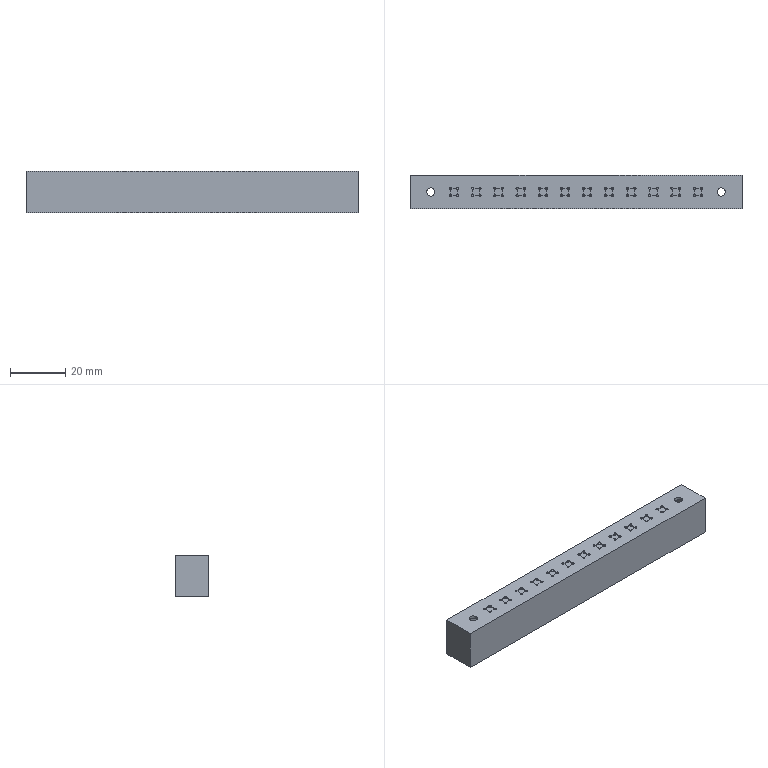Part | SolidWorks | features BaseBody 1 | 1 solid | 265 faces | box 120 x 12 x 15 mm | volume 9058 mm3 | cone 108 | cylinder 86 | plane 71 | commonest cylinder face diameters 0.8 x72 2 x6 1.567 x4 3 x4